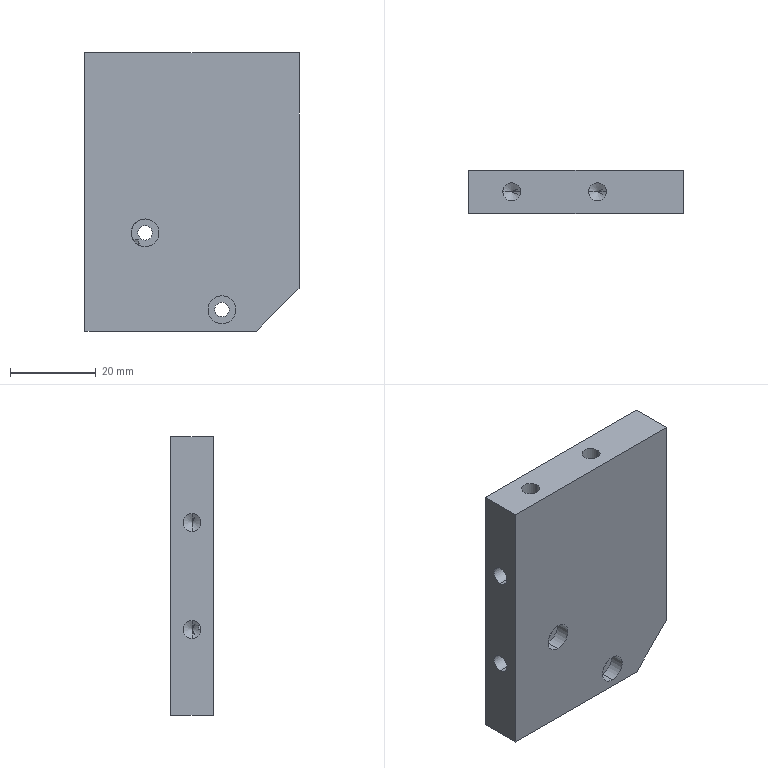Part | SolidWorks | features HoleWzd 3, Chamfer 2, Extrusion 1, ICE 1 | 1 solid | 33 faces | box 50 x 10 x 65 mm | volume 30944 mm3 | cylinder 16 | plane 9 | cone 8 | commonest cylinder face diameters 4.2 x8 3.4 x4 6.5 x4
STEP:
#1=CARTESIAN_POINT('',(-17.1,0.,20.1));
#2=VERTEX_POINT('',#1);
#3=CARTESIAN_POINT('',(-12.9,0.,20.1));
#4=VERTEX_POINT('',#3);
#5=CARTESIAN_POINT('',(-15.,0.,20.1));
#6=DIRECTION('',(0.,0.,1.));
#7=DIRECTION('',(1.,0.,0.));
#8=AXIS2_PLACEMENT_3D('',#5,#6,#7);
#9=CIRCLE('',#8,2.1);
#10=EDGE_CURVE('',#2,#4,#9,.T.);
#11=ORIENTED_EDGE('',*,*,#10,.F.);
#12=CARTESIAN_POINT('',(-17.1,0.,32.5));
#13=VERTEX_POINT('',#12);
#14=CARTESIAN_POINT('',(-17.1,0.,32.5));
#15=DIRECTION('',(0.,0.,1.));
#16=VECTOR('',#15,1000.);
#17=LINE('',#14,#16);
#18=EDGE_CURVE('',#2,#13,#17,.T.);
#19=ORIENTED_EDGE('',*,*,#18,.T.);
#20=CARTESIAN_POINT('',(-12.9,0.,32.5));
#21=VERTEX_POINT('',#20);
#22=CARTESIAN_POINT('',(-15.,0.,32.5));
#23=DIRECTION('',(0.,0.,1.));
#24=DIRECTION('',(1.,0.,0.));
#25=AXIS2_PLACEMENT_3D('',#22,#23,#24);
#26=CIRCLE('',#25,2.1);
#27=EDGE_CURVE('',#13,#21,#26,.T.);
#28=ORIENTED_EDGE('',*,*,#27,.T.);
#29=CARTESIAN_POINT('',(-12.9,0.,32.5));
#30=DIRECTION('',(0.,0.,1.));
#31=VECTOR('',#30,1000.);
#32=LINE('',#29,#31);
#33=EDGE_CURVE('',#4,#21,#32,.T.);
#34=ORIENTED_EDGE('',*,*,#33,.F.);
#35=EDGE_LOOP('',(#11,#19,#28,#34));
#36=FACE_OUTER_BOUND('',#35,.T.);
#37=CARTESIAN_POINT('',(-15.,0.,32.5));
#38=DIRECTION('',(0.,0.,1.));
#39=DIRECTION('',(1.,0.,0.));
#40=AXIS2_PLACEMENT_3D('',#37,#38,#39);
#41=CYLINDRICAL_SURFACE('',#40,2.1);
#42=ADVANCED_FACE('',(#36),#41,.F.);
#43=CARTESIAN_POINT('',(-15.,0.,18.838));
#44=VERTEX_POINT('',#43);
#45=CARTESIAN_POINT('',(-12.9,0.,20.1));
#46=DIRECTION('',(0.8572,0.,0.515));
#47=VECTOR('',#46,1000.);
#48=LINE('',#45,#47);
#49=EDGE_CURVE('',#44,#4,#48,.T.);
#50=ORIENTED_EDGE('',*,*,#49,.F.);
#51=CARTESIAN_POINT('',(-17.1,0.,20.1));
#52=DIRECTION('',(-0.8572,0.,0.515));
#53=VECTOR('',#52,1000.);
#54=LINE('',#51,#53);
#55=EDGE_CURVE('',#44,#2,#54,.T.);
#56=ORIENTED_EDGE('',*,*,#55,.T.);
#57=ORIENTED_EDGE('',*,*,#10,.T.);
#58=EDGE_LOOP('',(#50,#56,#57));
#59=FACE_OUTER_BOUND('',#58,.T.);
#60=CARTESIAN_POINT('',(-15.,0.,20.1));
#61=DIRECTION('',(0.,0.,1.));
#62=DIRECTION('',(1.,0.,0.));
#63=AXIS2_PLACEMENT_3D('',#60,#61,#62);
#64=CONICAL_SURFACE('',#63,2.1,1.03);
#65=ADVANCED_FACE('',(#59),#64,.F.);
#66=CARTESIAN_POINT('',(2.9,0.,20.1));
#67=VERTEX_POINT('',#66);
#68=CARTESIAN_POINT('',(7.1,0.,20.1));
#69=VERTEX_POINT('',#68);
#70=CARTESIAN_POINT('',(5.,0.,20.1));
#71=DIRECTION('',(0.,0.,1.));
#72=DIRECTION('',(1.,0.,0.));
#73=AXIS2_PLACEMENT_3D('',#70,#71,#72);
#74=CIRCLE('',#73,2.1);
#75=EDGE_CURVE('',#67,#69,#74,.T.);
#76=ORIENTED_EDGE('',*,*,#75,.F.);
#77=CARTESIAN_POINT('',(2.9,0.,32.5));
#78=VERTEX_POINT('',#77);
#79=CARTESIAN_POINT('',(2.9,0.,32.5));
#80=DIRECTION('',(0.,0.,1.));
#81=VECTOR('',#80,1000.);
#82=LINE('',#79,#81);
#83=EDGE_CURVE('',#67,#78,#82,.T.);
#84=ORIENTED_EDGE('',*,*,#83,.T.);
#85=CARTESIAN_POINT('',(7.1,0.,32.5));
#86=VERTEX_POINT('',#85);
#87=CARTESIAN_POINT('',(5.,0.,32.5));
#88=DIRECTION('',(0.,0.,1.));
#89=DIRECTION('',(1.,0.,0.));
#90=AXIS2_PLACEMENT_3D('',#87,#88,#89);
#91=CIRCLE('',#90,2.1);
#92=EDGE_CURVE('',#78,#86,#91,.T.);
#93=ORIENTED_EDGE('',*,*,#92,.T.);
#94=CARTESIAN_POINT('',(7.1,0.,32.5));
#95=DIRECTION('',(0.,0.,1.));
#96=VECTOR('',#95,1000.);
#97=LINE('',#94,#96);
#98=EDGE_CURVE('',#69,#86,#97,.T.);
#99=ORIENTED_EDGE('',*,*,#98,.F.);
#100=EDGE_LOOP('',(#76,#84,#93,#99));
#101=FACE_OUTER_BOUND('',#100,.T.);
#102=CARTESIAN_POINT('',(5.,0.,32.5));
#103=DIRECTION('',(0.,0.,1.));
#104=DIRECTION('',(1.,0.,0.));
#105=AXIS2_PLACEMENT_3D('',#102,#103,#104);
#106=CYLINDRICAL_SURFACE('',#105,2.1);
#107=ADVANCED_FACE('',(#101),#106,.F.);
#108=CARTESIAN_POINT('',(5.,0.,18.838));
#109=VERTEX_POINT('',#108);
#110=CARTESIAN_POINT('',(7.1,0.,20.1));
#111=DIRECTION('',(0.8572,0.,0.515));
#112=VECTOR('',#111,1000.);
#113=LINE('',#110,#112);
#114=EDGE_CURVE('',#109,#69,#113,.T.);
#115=ORIENTED_EDGE('',*,*,#114,.F.);
#116=CARTESIAN_POINT('',(2.9,0.,20.1));
#117=DIRECTION('',(-0.8572,0.,0.515));
#118=VECTOR('',#117,1000.);
#119=LINE('',#116,#118);
#120=EDGE_CURVE('',#109,#67,#119,.T.);
#121=ORIENTED_EDGE('',*,*,#120,.T.);
#122=ORIENTED_EDGE('',*,*,#75,.T.);
#123=EDGE_LOOP('',(#115,#121,#122));
#124=FACE_OUTER_BOUND('',#123,.T.);
#125=CARTESIAN_POINT('',(5.,0.,20.1));
#126=DIRECTION('',(0.,0.,1.));
#127=DIRECTION('',(1.,0.,0.));
#128=AXIS2_PLACEMENT_3D('',#125,#126,#127);
#129=CONICAL_SURFACE('',#128,2.1,1.03);
#130=ADVANCED_FACE('',(#124),#129,.F.);
#131=CARTESIAN_POINT('',(7.,-1.6,-24.25));
#132=VERTEX_POINT('',#131);
#133=CARTESIAN_POINT('',(7.,-1.6,-30.75));
#134=VERTEX_POINT('',#133);
#135=CARTESIAN_POINT('',(7.,-1.6,-27.5));
#136=DIRECTION('',(0.,-1.,0.));
#137=DIRECTION('',(0.,0.,-1.));
#138=AXIS2_PLACEMENT_3D('',#135,#136,#137);
#139=CIRCLE('',#138,3.25);
#140=EDGE_CURVE('',#132,#134,#139,.T.);
#141=ORIENTED_EDGE('',*,*,#140,.F.);
#142=CARTESIAN_POINT('',(7.,-5.,-24.25));
#143=VERTEX_POINT('',#142);
#144=CARTESIAN_POINT('',(7.,-5.,-24.25));
#145=DIRECTION('',(0.,-1.,0.));
#146=VECTOR('',#145,1000.);
#147=LINE('',#144,#146);
#148=EDGE_CURVE('',#132,#143,#147,.T.);
#149=ORIENTED_EDGE('',*,*,#148,.T.);
#150=CARTESIAN_POINT('',(7.,-5.,-30.75));
#151=VERTEX_POINT('',#150);
#152=CARTESIAN_POINT('',(7.,-5.,-27.5));
#153=DIRECTION('',(0.,-1.,0.));
#154=DIRECTION('',(0.,0.,-1.));
#155=AXIS2_PLACEMENT_3D('',#152,#153,#154);
#156=CIRCLE('',#155,3.25);
#157=EDGE_CURVE('',#143,#151,#156,.T.);
#158=ORIENTED_EDGE('',*,*,#157,.T.);
#159=CARTESIAN_POINT('',(7.,-5.,-30.75));
#160=DIRECTION('',(0.,-1.,0.));
#161=VECTOR('',#160,1000.);
#162=LINE('',#159,#161);
#163=EDGE_CURVE('',#134,#151,#162,.T.);
#164=ORIENTED_EDGE('',*,*,#163,.F.);
#165=EDGE_LOOP('',(#141,#149,#158,#164));
#166=FACE_OUTER_BOUND('',#165,.T.);
#167=CARTESIAN_POINT('',(7.,-5.,-27.5));
#168=DIRECTION('',(0.,-1.,0.));
#169=DIRECTION('',(0.,0.,-1.));
#170=AXIS2_PLACEMENT_3D('',#167,#168,#169);
#171=CYLINDRICAL_SURFACE('',#170,3.25);
#172=ADVANCED_FACE('',(#166),#171,.F.);
#173=CARTESIAN_POINT('',(7.,5.,-25.8));
#174=VERTEX_POINT('',#173);
#175=CARTESIAN_POINT('',(7.,5.,-29.2));
#176=VERTEX_POINT('',#175);
#177=CARTESIAN_POINT('',(7.,5.,-27.5));
#178=DIRECTION('',(0.,-1.,0.));
#179=DIRECTION('',(0.,0.,-1.));
#180=AXIS2_PLACEMENT_3D('',#177,#178,#179);
#181=CIRCLE('',#180,1.7);
#182=EDGE_CURVE('',#174,#176,#181,.T.);
#183=ORIENTED_EDGE('',*,*,#182,.F.);
#184=CARTESIAN_POINT('',(7.,-1.6,-25.8));
#185=VERTEX_POINT('',#184);
#186=CARTESIAN_POINT('',(7.,-5.,-25.8));
#187=DIRECTION('',(0.,-1.,0.));
#188=VECTOR('',#187,1000.);
#189=LINE('',#186,#188);
#190=EDGE_CURVE('',#174,#185,#189,.T.);
#191=ORIENTED_EDGE('',*,*,#190,.T.);
#192=CARTESIAN_POINT('',(7.,-1.6,-29.2));
#193=VERTEX_POINT('',#192);
#194=CARTESIAN_POINT('',(7.,-1.6,-27.5));
#195=DIRECTION('',(0.,-1.,0.));
#196=DIRECTION('',(0.,0.,-1.));
#197=AXIS2_PLACEMENT_3D('',#194,#195,#196);
#198=CIRCLE('',#197,1.7);
#199=EDGE_CURVE('',#185,#193,#198,.T.);
#200=ORIENTED_EDGE('',*,*,#199,.T.);
#201=CARTESIAN_POINT('',(7.,-5.,-29.2));
#202=DIRECTION('',(0.,-1.,0.));
#203=VECTOR('',#202,1000.);
#204=LINE('',#201,#203);
#205=EDGE_CURVE('',#176,#193,#204,.T.);
#206=ORIENTED_EDGE('',*,*,#205,.F.);
#207=EDGE_LOOP('',(#183,#191,#200,#206));
#208=FACE_OUTER_BOUND('',#207,.T.);
#209=CARTESIAN_POINT('',(7.,-5.,-27.5));
#210=DIRECTION('',(0.,-1.,0.));
#211=DIRECTION('',(0.,0.,-1.));
#212=AXIS2_PLACEMENT_3D('',#209,#210,#211);
#213=CYLINDRICAL_SURFACE('',#212,1.7);
#214=ADVANCED_FACE('',(#208),#213,.F.);
#215=CARTESIAN_POINT('',(-10.961,5.,-7.839));
#216=VERTEX_POINT('',#215);
#217=CARTESIAN_POINT('',(-10.961,5.,-11.239));
#218=VERTEX_POINT('',#217);
#219=CARTESIAN_POINT('',(-10.961,5.,-9.539));
#220=DIRECTION('',(0.,-1.,0.));
#221=DIRECTION('',(0.,0.,-1.));
#222=AXIS2_PLACEMENT_3D('',#219,#220,#221);
#223=CIRCLE('',#222,1.7);
#224=EDGE_CURVE('',#216,#218,#223,.T.);
#225=ORIENTED_EDGE('',*,*,#224,.F.);
#226=CARTESIAN_POINT('',(-10.961,-1.6,-7.839));
#227=VERTEX_POINT('',#226);
#228=CARTESIAN_POINT('',(-10.961,-5.,-7.839));
#229=DIRECTION('',(0.,-1.,0.));
#230=VECTOR('',#229,1000.);
#231=LINE('',#228,#230);
#232=EDGE_CURVE('',#216,#227,#231,.T.);
#233=ORIENTED_EDGE('',*,*,#232,.T.);
#234=CARTESIAN_POINT('',(-10.961,-1.6,-11.239));
#235=VERTEX_POINT('',#234);
#236=CARTESIAN_POINT('',(-10.961,-1.6,-9.539));
#237=DIRECTION('',(0.,-1.,0.));
#238=DIRECTION('',(0.,0.,-1.));
#239=AXIS2_PLACEMENT_3D('',#236,#237,#238);
#240=CIRCLE('',#239,1.7);
#241=EDGE_CURVE('',#227,#235,#240,.T.);
#242=ORIENTED_EDGE('',*,*,#241,.T.);
#243=CARTESIAN_POINT('',(-10.961,-5.,-11.239));
#244=DIRECTION('',(0.,-1.,0.));
#245=VECTOR('',#244,1000.);
#246=LINE('',#243,#245);
#247=EDGE_CURVE('',#218,#235,#246,.T.);
#248=ORIENTED_EDGE('',*,*,#247,.F.);
#249=EDGE_LOOP('',(#225,#233,#242,#248));
#250=FACE_OUTER_BOUND('',#249,.T.);
#251=CARTESIAN_POINT('',(-10.961,-5.,-9.539));
#252=DIRECTION('',(0.,-1.,0.));
#253=DIRECTION('',(0.,0.,-1.));
#254=AXIS2_PLACEMENT_3D('',#251,#252,#253);
#255=CYLINDRICAL_SURFACE('',#254,1.7);
#256=ADVANCED_FACE('',(#250),#255,.F.);
#257=CARTESIAN_POINT('',(-10.961,-1.6,-6.289));
#258=VERTEX_POINT('',#257);
#259=CARTESIAN_POINT('',(-13.789,-1.6,-11.14));
#260=VERTEX_POINT('',#259);
#261=CARTESIAN_POINT('',(-10.961,-1.6,-9.539));
#262=DIRECTION('',(0.,-1.,0.));
#263=DIRECTION('',(0.,0.,-1.));
#264=AXIS2_PLACEMENT_3D('',#261,#262,#263);
#265=CIRCLE('',#264,3.25);
#266=EDGE_CURVE('',#258,#260,#265,.T.);
#267=ORIENTED_EDGE('',*,*,#266,.F.);
#268=CARTESIAN_POINT('',(-10.961,-5.,-6.289));
#269=VERTEX_POINT('',#268);
#270=CARTESIAN_POINT('',(-10.961,-5.,-6.289));
#271=DIRECTION('',(0.,-1.,0.));
#272=VECTOR('',#271,1000.);
#273=LINE('',#270,#272);
#274=EDGE_CURVE('',#258,#269,#273,.T.);
#275=ORIENTED_EDGE('',*,*,#274,.T.);
#276=CARTESIAN_POINT('',(-10.961,-5.,-12.789));
#277=VERTEX_POINT('',#276);
#278=CARTESIAN_POINT('',(-10.961,-5.,-9.539));
#279=DIRECTION('',(0.,-1.,0.));
#280=DIRECTION('',(0.,0.,-1.));
#281=AXIS2_PLACEMENT_3D('',#278,#279,#280);
#282=CIRCLE('',#281,3.25);
#283=EDGE_CURVE('',#269,#277,#282,.T.);
#284=ORIENTED_EDGE('',*,*,#283,.T.);
#285=CARTESIAN_POINT('',(-10.961,-1.6,-12.789));
#286=VERTEX_POINT('',#285);
#287=CARTESIAN_POINT('',(-10.961,-5.,-12.789));
#288=DIRECTION('',(0.,-1.,0.));
#289=VECTOR('',#288,1000.);
#290=LINE('',#287,#289);
#291=EDGE_CURVE('',#286,#277,#290,.T.);
#292=ORIENTED_EDGE('',*,*,#291,.F.);
#293=CARTESIAN_POINT('',(-12.3,-1.6,-12.501));
#294=VERTEX_POINT('',#293);
#295=CARTESIAN_POINT('',(-10.961,-1.6,-9.539));
#296=DIRECTION('',(0.,-1.,0.));
#297=DIRECTION('',(0.,0.,-1.));
#298=AXIS2_PLACEMENT_3D('',#295,#296,#297);
#299=CIRCLE('',#298,3.25);
#300=EDGE_CURVE('',#294,#286,#299,.T.);
#301=ORIENTED_EDGE('',*,*,#300,.F.);
#302=CARTESIAN_POINT('',(-12.6,-2.094,-12.346));
#303=VERTEX_POINT('',#302);
#304=CARTESIAN_POINT('',(-12.6,-2.094,-12.346));
#305=CARTESIAN_POINT('',(-12.5,-1.932,-12.404));
#306=CARTESIAN_POINT('',(-12.4,-1.767,-12.456));
#307=CARTESIAN_POINT('',(-12.3,-1.6,-12.501));
#308=B_SPLINE_CURVE_WITH_KNOTS('',3,(#304,#305,#306,#307),.UNSPECIFIED.,.F.,.F.,(4,4),(0.00006868,0.0006676),.UNSPECIFIED.);
#309=EDGE_CURVE('',#303,#294,#308,.T.);
#310=ORIENTED_EDGE('',*,*,#309,.F.);
#311=CARTESIAN_POINT('',(-13.789,-1.6,-11.14));
#312=CARTESIAN_POINT('',(-13.729,-1.691,-11.246));
#313=CARTESIAN_POINT('',(-13.659,-1.766,-11.356));
#314=CARTESIAN_POINT('',(-13.497,-1.89,-11.576));
#315=CARTESIAN_POINT('',(-13.404,-1.94,-11.687));
#316=CARTESIAN_POINT('',(-13.101,-2.052,-12.003));
#317=CARTESIAN_POINT('',(-12.862,-2.083,-12.193));
#318=CARTESIAN_POINT('',(-12.6,-2.094,-12.346));
#319=B_SPLINE_CURVE_WITH_KNOTS('',3,(#311,#312,#313,#314,#315,#316,#317,#318),.UNSPECIFIED.,.F.,.F.,(4,2,2,4),(0.,0.0004495,0.000899,0.001798),.UNSPECIFIED.);
#320=EDGE_CURVE('',#260,#303,#319,.T.);
#321=ORIENTED_EDGE('',*,*,#320,.F.);
#322=EDGE_LOOP('',(#267,#275,#284,#292,#301,#310,#321));
#323=FACE_OUTER_BOUND('',#322,.T.);
#324=CARTESIAN_POINT('',(-10.961,-5.,-9.539));
#325=DIRECTION('',(0.,-1.,0.));
#326=DIRECTION('',(0.,0.,-1.));
#327=AXIS2_PLACEMENT_3D('',#324,#325,#326);
#328=CYLINDRICAL_SURFACE('',#327,3.25);
#329=ADVANCED_FACE('',(#323),#328,.F.);
#330=CARTESIAN_POINT('',(-12.6,0.,-14.6));
#331=VERTEX_POINT('',#330);
#332=CARTESIAN_POINT('',(-12.6,0.,-12.5));
#333=DIRECTION('',(-1.,0.,0.));
#334=DIRECTION('',(0.,0.,1.));
#335=AXIS2_PLACEMENT_3D('',#332,#333,#334);
#336=CIRCLE('',#335,2.1);
#337=EDGE_CURVE('',#331,#303,#336,.T.);
#338=ORIENTED_EDGE('',*,*,#337,.F.);
#339=CARTESIAN_POINT('',(-25.,0.,-14.6));
#340=VERTEX_POINT('',#339);
#341=CARTESIAN_POINT('',(-25.,0.,-14.6));
#342=DIRECTION('',(-1.,0.,0.));
#343=VECTOR('',#342,1000.);
#344=LINE('',#341,#343);
#345=EDGE_CURVE('',#331,#340,#344,.T.);
#346=ORIENTED_EDGE('',*,*,#345,.T.);
#347=CARTESIAN_POINT('',(-25.,0.,-10.4));
#348=VERTEX_POINT('',#347);
#349=CARTESIAN_POINT('',(-25.,0.,-12.5));
#350=DIRECTION('',(-1.,0.,0.));
#351=DIRECTION('',(0.,0.,1.));
#352=AXIS2_PLACEMENT_3D('',#349,#350,#351);
#353=CIRCLE('',#352,2.1);
#354=EDGE_CURVE('',#340,#348,#353,.T.);
#355=ORIENTED_EDGE('',*,*,#354,.T.);
#356=CARTESIAN_POINT('',(-12.6,0.,-10.4));
#357=VERTEX_POINT('',#356);
#358=CARTESIAN_POINT('',(-25.,0.,-10.4));
#359=DIRECTION('',(-1.,0.,0.));
#360=VECTOR('',#359,1000.);
#361=LINE('',#358,#360);
#362=EDGE_CURVE('',#357,#348,#361,.T.);
#363=ORIENTED_EDGE('',*,*,#362,.F.);
#364=CARTESIAN_POINT('',(-12.6,-1.6,-11.14));
#365=VERTEX_POINT('',#364);
#366=CARTESIAN_POINT('',(-12.6,0.,-12.5));
#367=DIRECTION('',(-1.,0.,0.));
#368=DIRECTION('',(0.,0.,1.));
#369=AXIS2_PLACEMENT_3D('',#366,#367,#368);
#370=CIRCLE('',#369,2.1);
#371=EDGE_CURVE('',#365,#357,#370,.T.);
#372=ORIENTED_EDGE('',*,*,#371,.F.);
#373=CARTESIAN_POINT('',(-25.,-1.6,-11.14));
#374=DIRECTION('',(-1.,0.,0.));
#375=VECTOR('',#374,1000.);
#376=LINE('',#373,#375);
#377=EDGE_CURVE('',#365,#260,#376,.T.);
#378=ORIENTED_EDGE('',*,*,#377,.T.);
#379=ORIENTED_EDGE('',*,*,#320,.T.);
#380=EDGE_LOOP('',(#338,#346,#355,#363,#372,#378,#379));
#381=FACE_OUTER_BOUND('',#380,.T.);
#382=CARTESIAN_POINT('',(-25.,0.,-12.5));
#383=DIRECTION('',(-1.,0.,0.));
#384=DIRECTION('',(0.,0.,1.));
#385=AXIS2_PLACEMENT_3D('',#382,#383,#384);
#386=CYLINDRICAL_SURFACE('',#385,2.1);
#387=ADVANCED_FACE('',(#381),#386,.F.);
#388=CARTESIAN_POINT('',(-11.338,0.,-12.5));
#389=VERTEX_POINT('',#388);
#390=CARTESIAN_POINT('',(-12.6,0.,-10.4));
#391=DIRECTION('',(-0.515,0.,0.8572));
#392=VECTOR('',#391,1000.);
#393=LINE('',#390,#392);
#394=EDGE_CURVE('',#389,#357,#393,.T.);
#395=ORIENTED_EDGE('',*,*,#394,.F.);
#396=CARTESIAN_POINT('',(-12.6,0.,-14.6));
#397=DIRECTION('',(-0.515,0.,-0.8572));
#398=VECTOR('',#397,1000.);
#399=LINE('',#396,#398);
#400=EDGE_CURVE('',#389,#331,#399,.T.);
#401=ORIENTED_EDGE('',*,*,#400,.T.);
#402=ORIENTED_EDGE('',*,*,#337,.T.);
#403=ORIENTED_EDGE('',*,*,#309,.T.);
#404=CARTESIAN_POINT('',(-12.3,-1.6,-12.501));
#405=CARTESIAN_POINT('',(-12.299,-1.6,-12.03));
#406=CARTESIAN_POINT('',(-12.431,-1.6,-11.573));
#407=CARTESIAN_POINT('',(-12.6,-1.6,-11.14));
#408=B_SPLINE_CURVE_WITH_KNOTS('',3,(#404,#405,#406,#407),.UNSPECIFIED.,.F.,.F.,(4,4),(0.0043,0.005691),.UNSPECIFIED.);
#409=EDGE_CURVE('',#294,#365,#408,.T.);
#410=ORIENTED_EDGE('',*,*,#409,.T.);
#411=ORIENTED_EDGE('',*,*,#371,.T.);
#412=EDGE_LOOP('',(#395,#401,#402,#403,#410,#411));
#413=FACE_OUTER_BOUND('',#412,.T.);
#414=CARTESIAN_POINT('',(-12.6,0.,-12.5));
#415=DIRECTION('',(-1.,0.,0.));
#416=DIRECTION('',(0.,0.,1.));
#417=AXIS2_PLACEMENT_3D('',#414,#415,#416);
#418=CONICAL_SURFACE('',#417,2.1,1.03);
#419=ADVANCED_FACE('',(#413),#418,.F.);
#420=CARTESIAN_POINT('',(-12.6,0.,10.4));
#421=VERTEX_POINT('',#420);
#422=CARTESIAN_POINT('',(-12.6,0.,14.6));
#423=VERTEX_POINT('',#422);
#424=CARTESIAN_POINT('',(-12.6,0.,12.5));
#425=DIRECTION('',(-1.,0.,0.));
#426=DIRECTION('',(0.,0.,1.));
#427=AXIS2_PLACEMENT_3D('',#424,#425,#426);
#428=CIRCLE('',#427,2.1);
#429=EDGE_CURVE('',#421,#423,#428,.T.);
#430=ORIENTED_EDGE('',*,*,#429,.F.);
#431=CARTESIAN_POINT('',(-25.,0.,10.4));
#432=VERTEX_POINT('',#431);
#433=CARTESIAN_POINT('',(-25.,0.,10.4));
#434=DIRECTION('',(-1.,0.,0.));
#435=VECTOR('',#434,1000.);
#436=LINE('',#433,#435);
#437=EDGE_CURVE('',#421,#432,#436,.T.);
#438=ORIENTED_EDGE('',*,*,#437,.T.);
#439=CARTESIAN_POINT('',(-25.,0.,14.6));
#440=VERTEX_POINT('',#439);
#441=CARTESIAN_POINT('',(-25.,0.,12.5));
#442=DIRECTION('',(-1.,0.,0.));
#443=DIRECTION('',(0.,0.,1.));
#444=AXIS2_PLACEMENT_3D('',#441,#442,#443);
#445=CIRCLE('',#444,2.1);
#446=EDGE_CURVE('',#432,#440,#445,.T.);
#447=ORIENTED_EDGE('',*,*,#446,.T.);
#448=CARTESIAN_POINT('',(-25.,0.,14.6));
#449=DIRECTION('',(-1.,0.,0.));
#450=VECTOR('',#449,1000.);
#451=LINE('',#448,#450);
#452=EDGE_CURVE('',#423,#440,#451,.T.);
#453=ORIENTED_EDGE('',*,*,#452,.F.);
#454=EDGE_LOOP('',(#430,#438,#447,#453));
#455=FACE_OUTER_BOUND('',#454,.T.);
#456=CARTESIAN_POINT('',(-25.,0.,12.5));
#457=DIRECTION('',(-1.,0.,0.));
#458=DIRECTION('',(0.,0.,1.));
#459=AXIS2_PLACEMENT_3D('',#456,#457,#458);
#460=CYLINDRICAL_SURFACE('',#459,2.1);
#461=ADVANCED_FACE('',(#455),#460,.F.);
#462=CARTESIAN_POINT('',(-11.338,0.,12.5));
#463=VERTEX_POINT('',#462);
#464=CARTESIAN_POINT('',(-12.6,0.,14.6));
#465=DIRECTION('',(-0.515,0.,0.8572));
#466=VECTOR('',#465,1000.);
#467=LINE('',#464,#466);
#468=EDGE_CURVE('',#463,#423,#467,.T.);
#469=ORIENTED_EDGE('',*,*,#468,.F.);
#470=CARTESIAN_POINT('',(-12.6,0.,10.4));
#471=DIRECTION('',(-0.515,0.,-0.8572));
#472=VECTOR('',#471,1000.);
#473=LINE('',#470,#472);
#474=EDGE_CURVE('',#463,#421,#473,.T.);
#475=ORIENTED_EDGE('',*,*,#474,.T.);
#476=ORIENTED_EDGE('',*,*,#429,.T.);
#477=EDGE_LOOP('',(#469,#475,#476));
#478=FACE_OUTER_BOUND('',#477,.T.);
#479=CARTESIAN_POINT('',(-12.6,0.,12.5));
#480=DIRECTION('',(-1.,0.,0.));
#481=DIRECTION('',(0.,0.,1.));
#482=AXIS2_PLACEMENT_3D('',#479,#480,#481);
#483=CONICAL_SURFACE('',#482,2.1,1.03);
#484=ADVANCED_FACE('',(#478),#483,.F.);
#485=CARTESIAN_POINT('',(25.,-5.,32.5));
#486=VERTEX_POINT('',#485);
#487=CARTESIAN_POINT('',(25.,-5.,-22.5));
#488=VERTEX_POINT('',#487);
#489=CARTESIAN_POINT('',(25.,-5.,-32.5));
#490=DIRECTION('',(0.,0.,-1.));
#491=VECTOR('',#490,1000.);
#492=LINE('',#489,#491);
#493=EDGE_CURVE('',#486,#488,#492,.T.);
#494=ORIENTED_EDGE('',*,*,#493,.T.);
#495=CARTESIAN_POINT('',(25.,5.,-22.5));
#496=VERTEX_POINT('',#495);
#497=CARTESIAN_POINT('',(25.,5.,-22.5));
#498=DIRECTION('',(0.,1.,0.));
#499=VECTOR('',#498,1000.);
#500=LINE('',#497,#499);
#501=EDGE_CURVE('',#488,#496,#500,.T.);
#502=ORIENTED_EDGE('',*,*,#501,.T.);
#503=CARTESIAN_POINT('',(25.,5.,32.5));
#504=VERTEX_POINT('',#503);
#505=CARTESIAN_POINT('',(25.,5.,-32.5));
#506=DIRECTION('',(0.,0.,-1.));
#507=VECTOR('',#506,1000.);
#508=LINE('',#505,#507);
#509=EDGE_CURVE('',#504,#496,#508,.T.);
#510=ORIENTED_EDGE('',*,*,#509,.F.);
#511=CARTESIAN_POINT('',(25.,5.,32.5));
#512=DIRECTION('',(0.,-1.,0.));
#513=VECTOR('',#512,1000.);
#514=LINE('',#511,#513);
#515=EDGE_CURVE('',#504,#486,#514,.T.);
#516=ORIENTED_EDGE('',*,*,#515,.T.);
#517=EDGE_LOOP('',(#494,#502,#510,#516));
#518=FACE_OUTER_BOUND('',#517,.T.);
#519=CARTESIAN_POINT('',(25.,5.,-32.5));
#520=DIRECTION('',(-1.,0.,0.));
#521=DIRECTION('',(0.,0.,1.));
#522=AXIS2_PLACEMENT_3D('',#519,#520,#521);
#523=PLANE('',#522);
#524=ADVANCED_FACE('',(#518),#523,.F.);
#525=CARTESIAN_POINT('',(15.,5.,-32.5));
#526=VERTEX_POINT('',#525);
#527=CARTESIAN_POINT('',(-25.,5.,-32.5));
#528=VERTEX_POINT('',#527);
#529=CARTESIAN_POINT('',(-25.,5.,-32.5));
#530=DIRECTION('',(-1.,0.,0.));
#531=VECTOR('',#530,1000.);
#532=LINE('',#529,#531);
#533=EDGE_CURVE('',#526,#528,#532,.T.);
#534=ORIENTED_EDGE('',*,*,#533,.F.);
#535=CARTESIAN_POINT('',(15.,-5.,-32.5));
#536=VERTEX_POINT('',#535);
#537=CARTESIAN_POINT('',(15.,5.,-32.5));
#538=DIRECTION('',(0.,-1.,0.));
#539=VECTOR('',#538,1000.);
#540=LINE('',#537,#539);
#541=EDGE_CURVE('',#526,#536,#540,.T.);
#542=ORIENTED_EDGE('',*,*,#541,.T.);
#543=CARTESIAN_POINT('',(-25.,-5.,-32.5));
#544=VERTEX_POINT('',#543);
#545=CARTESIAN_POINT('',(-25.,-5.,-32.5));
#546=DIRECTION('',(-1.,0.,0.));
#547=VECTOR('',#546,1000.);
#548=LINE('',#545,#547);
#549=EDGE_CURVE('',#536,#544,#548,.T.);
#550=ORIENTED_EDGE('',*,*,#549,.T.);
#551=CARTESIAN_POINT('',(-25.,5.,-32.5));
#552=DIRECTION('',(0.,-1.,0.));
#553=VECTOR('',#552,1000.);
#554=LINE('',#551,#553);
#555=EDGE_CURVE('',#528,#544,#554,.T.);
#556=ORIENTED_EDGE('',*,*,#555,.F.);
#557=EDGE_LOOP('',(#534,#542,#550,#556));
#558=FACE_OUTER_BOUND('',#557,.T.);
#559=CARTESIAN_POINT('',(-25.,5.,-32.5));
#560=DIRECTION('',(0.,0.,1.));
#561=DIRECTION('',(1.,0.,0.));
#562=AXIS2_PLACEMENT_3D('',#559,#560,#561);
#563=PLANE('',#562);
#564=ADVANCED_FACE('',(#558),#563,.F.);
#565=CARTESIAN_POINT('',(-25.,0.,-12.5));
#566=DIRECTION('',(-1.,0.,0.));
#567=DIRECTION('',(0.,0.,1.));
#568=AXIS2_PLACEMENT_3D('',#565,#566,#567);
#569=CIRCLE('',#568,2.1);
#570=EDGE_CURVE('',#348,#340,#569,.T.);
#571=ORIENTED_EDGE('',*,*,#570,.F.);
#572=ORIENTED_EDGE('',*,*,#354,.F.);
#573=EDGE_LOOP('',(#571,#572));
#574=FACE_BOUND('',#573,.T.);
#575=CARTESIAN_POINT('',(-25.,0.,12.5));
#576=DIRECTION('',(-1.,0.,0.));
#577=DIRECTION('',(0.,0.,1.));
#578=AXIS2_PLACEMENT_3D('',#575,#576,#577);
#579=CIRCLE('',#578,2.1);
#580=EDGE_CURVE('',#440,#432,#579,.T.);
#581=ORIENTED_EDGE('',*,*,#580,.F.);
#582=ORIENTED_EDGE('',*,*,#446,.F.);
#583=EDGE_LOOP('',(#581,#582));
#584=FACE_BOUND('',#583,.T.);
#585=CARTESIAN_POINT('',(-25.,-5.,32.5));
#586=VERTEX_POINT('',#585);
#587=CARTESIAN_POINT('',(-25.,-5.,-32.5));
#588=DIRECTION('',(0.,0.,1.));
#589=VECTOR('',#588,1000.);
#590=LINE('',#587,#589);
#591=EDGE_CURVE('',#544,#586,#590,.T.);
#592=ORIENTED_EDGE('',*,*,#591,.T.);
#593=CARTESIAN_POINT('',(-25.,5.,32.5));
#594=VERTEX_POINT('',#593);
#595=CARTESIAN_POINT('',(-25.,5.,32.5));
#596=DIRECTION('',(0.,-1.,0.));
#597=VECTOR('',#596,1000.);
#598=LINE('',#595,#597);
#599=EDGE_CURVE('',#594,#586,#598,.T.);
#600=ORIENTED_EDGE('',*,*,#599,.F.);
#601=CARTESIAN_POINT('',(-25.,5.,-32.5));
#602=DIRECTION('',(0.,0.,1.));
#603=VECTOR('',#602,1000.);
#604=LINE('',#601,#603);
#605=EDGE_CURVE('',#528,#594,#604,.T.);
#606=ORIENTED_EDGE('',*,*,#605,.F.);
#607=ORIENTED_EDGE('',*,*,#555,.T.);
#608=EDGE_LOOP('',(#592,#600,#606,#607));
#609=FACE_OUTER_BOUND('',#608,.T.);
#610=CARTESIAN_POINT('',(-25.,5.,-32.5));
#611=DIRECTION('',(1.,0.,0.));
#612=DIRECTION('',(0.,0.,-1.));
#613=AXIS2_PLACEMENT_3D('',#610,#611,#612);
#614=PLANE('',#613);
#615=ADVANCED_FACE('',(#574,#584,#609),#614,.F.);
#616=CARTESIAN_POINT('',(-15.,0.,32.5));
#617=DIRECTION('',(0.,0.,1.));
#618=DIRECTION('',(1.,0.,0.));
#619=AXIS2_PLACEMENT_3D('',#616,#617,#618);
#620=CIRCLE('',#619,2.1);
#621=EDGE_CURVE('',#21,#13,#620,.T.);
#622=ORIENTED_EDGE('',*,*,#621,.F.);
#623=ORIENTED_EDGE('',*,*,#27,.F.);
#624=EDGE_LOOP('',(#622,#623));
#625=FACE_BOUND('',#624,.T.);
#626=CARTESIAN_POINT('',(5.,0.,32.5));
#627=DIRECTION('',(0.,0.,1.));
#628=DIRECTION('',(1.,0.,0.));
#629=AXIS2_PLACEMENT_3D('',#626,#627,#628);
#630=CIRCLE('',#629,2.1);
#631=EDGE_CURVE('',#86,#78,#630,.T.);
#632=ORIENTED_EDGE('',*,*,#631,.F.);
#633=ORIENTED_EDGE('',*,*,#92,.F.);
#634=EDGE_LOOP('',(#632,#633));
#635=FACE_BOUND('',#634,.T.);
#636=CARTESIAN_POINT('',(-25.,-5.,32.5));
#637=DIRECTION('',(1.,0.,0.));
#638=VECTOR('',#637,1000.);
#639=LINE('',#636,#638);
#640=EDGE_CURVE('',#586,#486,#639,.T.);
#641=ORIENTED_EDGE('',*,*,#640,.T.);
#642=ORIENTED_EDGE('',*,*,#515,.F.);
#643=CARTESIAN_POINT('',(-25.,5.,32.5));
#644=DIRECTION('',(1.,0.,0.));
#645=VECTOR('',#644,1000.);
#646=LINE('',#643,#645);
#647=EDGE_CURVE('',#594,#504,#646,.T.);
#648=ORIENTED_EDGE('',*,*,#647,.F.);
#649=ORIENTED_EDGE('',*,*,#599,.T.);
#650=EDGE_LOOP('',(#641,#642,#648,#649));
#651=FACE_OUTER_BOUND('',#650,.T.);
#652=CARTESIAN_POINT('',(-25.,5.,32.5));
#653=DIRECTION('',(0.,0.,-1.));
#654=DIRECTION('',(-1.,0.,0.));
#655=AXIS2_PLACEMENT_3D('',#652,#653,#654);
#656=PLANE('',#655);
#657=ADVANCED_FACE('',(#625,#635,#651),#656,.F.);
#658=CARTESIAN_POINT('',(7.,5.,-27.5));
#659=DIRECTION('',(0.,-1.,0.));
#660=DIRECTION('',(0.,0.,-1.));
#661=AXIS2_PLACEMENT_3D('',#658,#659,#660);
#662=CIRCLE('',#661,1.7);
#663=EDGE_CURVE('',#176,#174,#662,.T.);
#664=ORIENTED_EDGE('',*,*,#663,.T.);
#665=ORIENTED_EDGE('',*,*,#182,.T.);
#666=EDGE_LOOP('',(#664,#665));
#667=FACE_BOUND('',#666,.T.);
#668=CARTESIAN_POINT('',(-10.961,5.,-9.539));
#669=DIRECTION('',(0.,-1.,0.));
#670=DIRECTION('',(0.,0.,-1.));
#671=AXIS2_PLACEMENT_3D('',#668,#669,#670);
#672=CIRCLE('',#671,1.7);
#673=EDGE_CURVE('',#218,#216,#672,.T.);
#674=ORIENTED_EDGE('',*,*,#673,.T.);
#675=ORIENTED_EDGE('',*,*,#224,.T.);
#676=EDGE_LOOP('',(#674,#675));
#677=FACE_BOUND('',#676,.T.);
#678=ORIENTED_EDGE('',*,*,#509,.T.);
#679=CARTESIAN_POINT('',(23.75,5.,-23.75));
#680=DIRECTION('',(-0.7071,0.,-0.7071));
#681=VECTOR('',#680,1000.);
#682=LINE('',#679,#681);
#683=EDGE_CURVE('',#496,#526,#682,.T.);
#684=ORIENTED_EDGE('',*,*,#683,.T.);
#685=ORIENTED_EDGE('',*,*,#533,.T.);
#686=ORIENTED_EDGE('',*,*,#605,.T.);
#687=ORIENTED_EDGE('',*,*,#647,.T.);
#688=EDGE_LOOP('',(#678,#684,#685,#686,#687));
#689=FACE_OUTER_BOUND('',#688,.T.);
#690=CARTESIAN_POINT('',(0.,5.,0.));
#691=DIRECTION('',(0.,1.,0.));
#692=DIRECTION('',(0.,0.,1.));
#693=AXIS2_PLACEMENT_3D('',#690,#691,#692);
#694=PLANE('',#693);
#695=ADVANCED_FACE('',(#667,#677,#689),#694,.T.);
#696=CARTESIAN_POINT('',(7.,-5.,-27.5));
#697=DIRECTION('',(0.,-1.,0.));
#698=DIRECTION('',(0.,0.,-1.));
#699=AXIS2_PLACEMENT_3D('',#696,#697,#698);
#700=CIRCLE('',#699,3.25);
#701=EDGE_CURVE('',#151,#143,#700,.T.);
#702=ORIENTED_EDGE('',*,*,#701,.F.);
#703=ORIENTED_EDGE('',*,*,#157,.F.);
#704=EDGE_LOOP('',(#702,#703));
#705=FACE_BOUND('',#704,.T.);
#706=CARTESIAN_POINT('',(-10.961,-5.,-9.539));
#707=DIRECTION('',(0.,-1.,0.));
#708=DIRECTION('',(0.,0.,-1.));
#709=AXIS2_PLACEMENT_3D('',#706,#707,#708);
#710=CIRCLE('',#709,3.25);
#711=EDGE_CURVE('',#277,#269,#710,.T.);
#712=ORIENTED_EDGE('',*,*,#711,.F.);
#713=ORIENTED_EDGE('',*,*,#283,.F.);
#714=EDGE_LOOP('',(#712,#713));
#715=FACE_BOUND('',#714,.T.);
#716=ORIENTED_EDGE('',*,*,#549,.F.);
#717=CARTESIAN_POINT('',(15.,-5.,-32.5));
#718=DIRECTION('',(0.7071,0.,0.7071));
#719=VECTOR('',#718,1000.);
#720=LINE('',#717,#719);
#721=EDGE_CURVE('',#536,#488,#720,.T.);
#722=ORIENTED_EDGE('',*,*,#721,.T.);
#723=ORIENTED_EDGE('',*,*,#493,.F.);
#724=ORIENTED_EDGE('',*,*,#640,.F.);
#725=ORIENTED_EDGE('',*,*,#591,.F.);
#726=EDGE_LOOP('',(#716,#722,#723,#724,#725));
#727=FACE_OUTER_BOUND('',#726,.T.);
#728=CARTESIAN_POINT('',(0.,-5.,0.));
#729=DIRECTION('',(0.,1.,0.));
#730=DIRECTION('',(0.,0.,1.));
#731=AXIS2_PLACEMENT_3D('',#728,#729,#730);
#732=PLANE('',#731);
#733=ADVANCED_FACE('',(#705,#715,#727),#732,.F.);
#734=ORIENTED_EDGE('',*,*,#683,.F.);
#735=ORIENTED_EDGE('',*,*,#501,.F.);
#736=ORIENTED_EDGE('',*,*,#721,.F.);
#737=ORIENTED_EDGE('',*,*,#541,.F.);
#738=EDGE_LOOP('',(#734,#735,#736,#737));
#739=FACE_OUTER_BOUND('',#738,.T.);
#740=CARTESIAN_POINT('',(15.,5.,-32.5));
#741=DIRECTION('',(-0.7071,0.,0.7071));
#742=DIRECTION('',(0.,-1.,0.));
#743=AXIS2_PLACEMENT_3D('',#740,#741,#742);
#744=PLANE('',#743);
#745=ADVANCED_FACE('',(#739),#744,.F.);
#746=ORIENTED_EDGE('',*,*,#474,.F.);
#747=ORIENTED_EDGE('',*,*,#468,.T.);
#748=CARTESIAN_POINT('',(-12.6,0.,12.5));
#749=DIRECTION('',(-1.,0.,0.));
#750=DIRECTION('',(0.,0.,1.));
#751=AXIS2_PLACEMENT_3D('',#748,#749,#750);
#752=CIRCLE('',#751,2.1);
#753=EDGE_CURVE('',#423,#421,#752,.T.);
#754=ORIENTED_EDGE('',*,*,#753,.T.);
#755=EDGE_LOOP('',(#746,#747,#754));
#756=FACE_OUTER_BOUND('',#755,.T.);
#757=CARTESIAN_POINT('',(-12.6,0.,12.5));
#758=DIRECTION('',(-1.,0.,0.));
#759=DIRECTION('',(0.,0.,1.));
#760=AXIS2_PLACEMENT_3D('',#757,#758,#759);
#761=CONICAL_SURFACE('',#760,2.1,1.03);
#762=ADVANCED_FACE('',(#756),#761,.F.);
#763=ORIENTED_EDGE('',*,*,#437,.F.);
#764=ORIENTED_EDGE('',*,*,#753,.F.);
#765=ORIENTED_EDGE('',*,*,#452,.T.);
#766=ORIENTED_EDGE('',*,*,#580,.T.);
#767=EDGE_LOOP('',(#763,#764,#765,#766));
#768=FACE_OUTER_BOUND('',#767,.T.);
#769=CARTESIAN_POINT('',(-25.,0.,12.5));
#770=DIRECTION('',(-1.,0.,0.));
#771=DIRECTION('',(0.,0.,1.));
#772=AXIS2_PLACEMENT_3D('',#769,#770,#771);
#773=CYLINDRICAL_SURFACE('',#772,2.1);
#774=ADVANCED_FACE('',(#768),#773,.F.);
#775=ORIENTED_EDGE('',*,*,#400,.F.);
#776=ORIENTED_EDGE('',*,*,#394,.T.);
#777=CARTESIAN_POINT('',(-12.6,0.,-12.5));
#778=DIRECTION('',(-1.,0.,0.));
#779=DIRECTION('',(0.,0.,1.));
#780=AXIS2_PLACEMENT_3D('',#777,#778,#779);
#781=CIRCLE('',#780,2.1);
#782=EDGE_CURVE('',#357,#331,#781,.T.);
#783=ORIENTED_EDGE('',*,*,#782,.T.);
#784=EDGE_LOOP('',(#775,#776,#783));
#785=FACE_OUTER_BOUND('',#784,.T.);
#786=CARTESIAN_POINT('',(-12.6,0.,-12.5));
#787=DIRECTION('',(-1.,0.,0.));
#788=DIRECTION('',(0.,0.,1.));
#789=AXIS2_PLACEMENT_3D('',#786,#787,#788);
#790=CONICAL_SURFACE('',#789,2.1,1.03);
#791=ADVANCED_FACE('',(#785),#790,.F.);
#792=ORIENTED_EDGE('',*,*,#345,.F.);
#793=ORIENTED_EDGE('',*,*,#782,.F.);
#794=ORIENTED_EDGE('',*,*,#362,.T.);
#795=ORIENTED_EDGE('',*,*,#570,.T.);
#796=EDGE_LOOP('',(#792,#793,#794,#795));
#797=FACE_OUTER_BOUND('',#796,.T.);
#798=CARTESIAN_POINT('',(-25.,0.,-12.5));
#799=DIRECTION('',(-1.,0.,0.));
#800=DIRECTION('',(0.,0.,1.));
#801=AXIS2_PLACEMENT_3D('',#798,#799,#800);
#802=CYLINDRICAL_SURFACE('',#801,2.1);
#803=ADVANCED_FACE('',(#797),#802,.F.);
#804=ORIENTED_EDGE('',*,*,#274,.F.);
#805=CARTESIAN_POINT('',(-10.961,-1.6,-9.539));
#806=DIRECTION('',(0.,-1.,0.));
#807=DIRECTION('',(0.,0.,-1.));
#808=AXIS2_PLACEMENT_3D('',#805,#806,#807);
#809=CIRCLE('',#808,3.25);
#810=EDGE_CURVE('',#286,#258,#809,.T.);
#811=ORIENTED_EDGE('',*,*,#810,.F.);
#812=ORIENTED_EDGE('',*,*,#291,.T.);
#813=ORIENTED_EDGE('',*,*,#711,.T.);
#814=EDGE_LOOP('',(#804,#811,#812,#813));
#815=FACE_OUTER_BOUND('',#814,.T.);
#816=CARTESIAN_POINT('',(-10.961,-5.,-9.539));
#817=DIRECTION('',(0.,-1.,0.));
#818=DIRECTION('',(0.,0.,-1.));
#819=AXIS2_PLACEMENT_3D('',#816,#817,#818);
#820=CYLINDRICAL_SURFACE('',#819,3.25);
#821=ADVANCED_FACE('',(#815),#820,.F.);
#822=CARTESIAN_POINT('',(-10.961,-1.6,-9.539));
#823=DIRECTION('',(0.,-1.,0.));
#824=DIRECTION('',(0.,0.,-1.));
#825=AXIS2_PLACEMENT_3D('',#822,#823,#824);
#826=CIRCLE('',#825,1.7);
#827=EDGE_CURVE('',#235,#227,#826,.T.);
#828=ORIENTED_EDGE('',*,*,#827,.F.);
#829=ORIENTED_EDGE('',*,*,#241,.F.);
#830=EDGE_LOOP('',(#828,#829));
#831=FACE_BOUND('',#830,.T.);
#832=ORIENTED_EDGE('',*,*,#409,.F.);
#833=ORIENTED_EDGE('',*,*,#300,.T.);
#834=ORIENTED_EDGE('',*,*,#810,.T.);
#835=ORIENTED_EDGE('',*,*,#266,.T.);
#836=ORIENTED_EDGE('',*,*,#377,.F.);
#837=EDGE_LOOP('',(#832,#833,#834,#835,#836));
#838=FACE_OUTER_BOUND('',#837,.T.);
#839=CARTESIAN_POINT('',(-9.261,-1.6,-9.539));
#840=DIRECTION('',(0.,1.,0.));
#841=DIRECTION('',(0.,0.,1.));
#842=AXIS2_PLACEMENT_3D('',#839,#840,#841);
#843=PLANE('',#842);
#844=ADVANCED_FACE('',(#831,#838),#843,.F.);
#845=ORIENTED_EDGE('',*,*,#232,.F.);
#846=ORIENTED_EDGE('',*,*,#673,.F.);
#847=ORIENTED_EDGE('',*,*,#247,.T.);
#848=ORIENTED_EDGE('',*,*,#827,.T.);
#849=EDGE_LOOP('',(#845,#846,#847,#848));
#850=FACE_OUTER_BOUND('',#849,.T.);
#851=CARTESIAN_POINT('',(-10.961,-5.,-9.539));
#852=DIRECTION('',(0.,-1.,0.));
#853=DIRECTION('',(0.,0.,-1.));
#854=AXIS2_PLACEMENT_3D('',#851,#852,#853);
#855=CYLINDRICAL_SURFACE('',#854,1.7);
#856=ADVANCED_FACE('',(#850),#855,.F.);
#857=ORIENTED_EDGE('',*,*,#190,.F.);
#858=ORIENTED_EDGE('',*,*,#663,.F.);
#859=ORIENTED_EDGE('',*,*,#205,.T.);
#860=CARTESIAN_POINT('',(7.,-1.6,-27.5));
#861=DIRECTION('',(0.,-1.,0.));
#862=DIRECTION('',(0.,0.,-1.));
#863=AXIS2_PLACEMENT_3D('',#860,#861,#862);
#864=CIRCLE('',#863,1.7);
#865=EDGE_CURVE('',#193,#185,#864,.T.);
#866=ORIENTED_EDGE('',*,*,#865,.T.);
#867=EDGE_LOOP('',(#857,#858,#859,#866));
#868=FACE_OUTER_BOUND('',#867,.T.);
#869=CARTESIAN_POINT('',(7.,-5.,-27.5));
#870=DIRECTION('',(0.,-1.,0.));
#871=DIRECTION('',(0.,0.,-1.));
#872=AXIS2_PLACEMENT_3D('',#869,#870,#871);
#873=CYLINDRICAL_SURFACE('',#872,1.7);
#874=ADVANCED_FACE('',(#868),#873,.F.);
#875=ORIENTED_EDGE('',*,*,#865,.F.);
#876=ORIENTED_EDGE('',*,*,#199,.F.);
#877=EDGE_LOOP('',(#875,#876));
#878=FACE_BOUND('',#877,.T.);
#879=CARTESIAN_POINT('',(7.,-1.6,-27.5));
#880=DIRECTION('',(0.,-1.,0.));
#881=DIRECTION('',(0.,0.,-1.));
#882=AXIS2_PLACEMENT_3D('',#879,#880,#881);
#883=CIRCLE('',#882,3.25);
#884=EDGE_CURVE('',#134,#132,#883,.T.);
#885=ORIENTED_EDGE('',*,*,#884,.T.);
#886=ORIENTED_EDGE('',*,*,#140,.T.);
#887=EDGE_LOOP('',(#885,#886));
#888=FACE_OUTER_BOUND('',#887,.T.);
#889=CARTESIAN_POINT('',(8.7,-1.6,-27.5));
#890=DIRECTION('',(0.,1.,0.));
#891=DIRECTION('',(0.,0.,1.));
#892=AXIS2_PLACEMENT_3D('',#889,#890,#891);
#893=PLANE('',#892);
#894=ADVANCED_FACE('',(#878,#888),#893,.F.);
#895=ORIENTED_EDGE('',*,*,#148,.F.);
#896=ORIENTED_EDGE('',*,*,#884,.F.);
#897=ORIENTED_EDGE('',*,*,#163,.T.);
#898=ORIENTED_EDGE('',*,*,#701,.T.);
#899=EDGE_LOOP('',(#895,#896,#897,#898));
#900=FACE_OUTER_BOUND('',#899,.T.);
#901=CARTESIAN_POINT('',(7.,-5.,-27.5));
#902=DIRECTION('',(0.,-1.,0.));
#903=DIRECTION('',(0.,0.,-1.));
#904=AXIS2_PLACEMENT_3D('',#901,#902,#903);
#905=CYLINDRICAL_SURFACE('',#904,3.25);
#906=ADVANCED_FACE('',(#900),#905,.F.);
#907=ORIENTED_EDGE('',*,*,#120,.F.);
#908=ORIENTED_EDGE('',*,*,#114,.T.);
#909=CARTESIAN_POINT('',(5.,0.,20.1));
#910=DIRECTION('',(0.,0.,1.));
#911=DIRECTION('',(1.,0.,0.));
#912=AXIS2_PLACEMENT_3D('',#909,#910,#911);
#913=CIRCLE('',#912,2.1);
#914=EDGE_CURVE('',#69,#67,#913,.T.);
#915=ORIENTED_EDGE('',*,*,#914,.T.);
#916=EDGE_LOOP('',(#907,#908,#915));
#917=FACE_OUTER_BOUND('',#916,.T.);
#918=CARTESIAN_POINT('',(5.,0.,20.1));
#919=DIRECTION('',(0.,0.,1.));
#920=DIRECTION('',(1.,0.,0.));
#921=AXIS2_PLACEMENT_3D('',#918,#919,#920);
#922=CONICAL_SURFACE('',#921,2.1,1.03);
#923=ADVANCED_FACE('',(#917),#922,.F.);
#924=ORIENTED_EDGE('',*,*,#83,.F.);
#925=ORIENTED_EDGE('',*,*,#914,.F.);
#926=ORIENTED_EDGE('',*,*,#98,.T.);
#927=ORIENTED_EDGE('',*,*,#631,.T.);
#928=EDGE_LOOP('',(#924,#925,#926,#927));
#929=FACE_OUTER_BOUND('',#928,.T.);
#930=CARTESIAN_POINT('',(5.,0.,32.5));
#931=DIRECTION('',(0.,0.,1.));
#932=DIRECTION('',(1.,0.,0.));
#933=AXIS2_PLACEMENT_3D('',#930,#931,#932);
#934=CYLINDRICAL_SURFACE('',#933,2.1);
#935=ADVANCED_FACE('',(#929),#934,.F.);
#936=ORIENTED_EDGE('',*,*,#55,.F.);
#937=ORIENTED_EDGE('',*,*,#49,.T.);
#938=CARTESIAN_POINT('',(-15.,0.,20.1));
#939=DIRECTION('',(0.,0.,1.));
#940=DIRECTION('',(1.,0.,0.));
#941=AXIS2_PLACEMENT_3D('',#938,#939,#940);
#942=CIRCLE('',#941,2.1);
#943=EDGE_CURVE('',#4,#2,#942,.T.);
#944=ORIENTED_EDGE('',*,*,#943,.T.);
#945=EDGE_LOOP('',(#936,#937,#944));
#946=FACE_OUTER_BOUND('',#945,.T.);
#947=CARTESIAN_POINT('',(-15.,0.,20.1));
#948=DIRECTION('',(0.,0.,1.));
#949=DIRECTION('',(1.,0.,0.));
#950=AXIS2_PLACEMENT_3D('',#947,#948,#949);
#951=CONICAL_SURFACE('',#950,2.1,1.03);
#952=ADVANCED_FACE('',(#946),#951,.F.);
#953=ORIENTED_EDGE('',*,*,#18,.F.);
#954=ORIENTED_EDGE('',*,*,#943,.F.);
#955=ORIENTED_EDGE('',*,*,#33,.T.);
#956=ORIENTED_EDGE('',*,*,#621,.T.);
#957=EDGE_LOOP('',(#953,#954,#955,#956));
#958=FACE_OUTER_BOUND('',#957,.T.);
#959=CARTESIAN_POINT('',(-15.,0.,32.5));
#960=DIRECTION('',(0.,0.,1.));
#961=DIRECTION('',(1.,0.,0.));
#962=AXIS2_PLACEMENT_3D('',#959,#960,#961);
#963=CYLINDRICAL_SURFACE('',#962,2.1);
#964=ADVANCED_FACE('',(#958),#963,.F.);
#965=CLOSED_SHELL('',(#42,#65,#107,#130,#172,#214,#256,#329,#387,#419,#461,#484,#524,#564,#615,#657,#695,#733,#745,#762,#774,#791,#803,#821,#844,#856,#874,#894,#906,#923,#935,#952,#964));
#966=MANIFOLD_SOLID_BREP('',#965);
#967=CARTESIAN_POINT('',(0.,0.,0.));
#968=DIRECTION('',(0.,0.,1.));
#969=DIRECTION('',(1.,0.,0.));
#970=AXIS2_PLACEMENT_3D('',#967,#968,#969);
#971=(LENGTH_UNIT()NAMED_UNIT(*)SI_UNIT(.MILLI.,.METRE.));
#972=UNCERTAINTY_MEASURE_WITH_UNIT(LENGTH_MEASURE(0.00001),#971,'','');
#973=(NAMED_UNIT(*)PLANE_ANGLE_UNIT()SI_UNIT($,.RADIAN.));
#974=(NAMED_UNIT(*)SI_UNIT($,.STERADIAN.)SOLID_ANGLE_UNIT());
#975=(GEOMETRIC_REPRESENTATION_CONTEXT(3)GLOBAL_UNCERTAINTY_ASSIGNED_CONTEXT((#972))GLOBAL_UNIT_ASSIGNED_CONTEXT((#971,#973,#974))REPRESENTATION_CONTEXT('',''));
#976=ADVANCED_BREP_SHAPE_REPRESENTATION('',(#966,#970),#975);